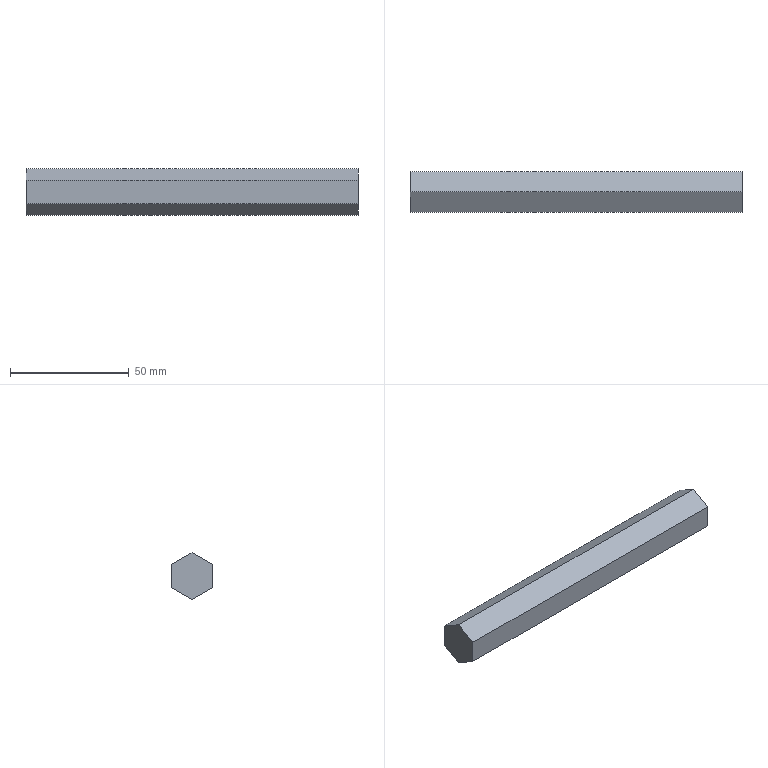Part | STEP file | JBJ-P-1002-09 | 1 solid | 8 faces | box 140 x 17 x 19.63 mm | volume 35039 mm3 | plane 8
STEP:
#1=CARTESIAN_POINT('',(0.,-8.5,4.907));
#2=VERTEX_POINT('',#1);
#3=CARTESIAN_POINT('',(0.,-8.5,-4.907));
#4=VERTEX_POINT('',#3);
#5=CARTESIAN_POINT('',(0.,-8.5,4.907));
#6=DIRECTION('',(0.,0.,-1.));
#7=VECTOR('',#6,1000.);
#8=LINE('',#5,#7);
#9=EDGE_CURVE('',#2,#4,#8,.T.);
#10=ORIENTED_EDGE('',*,*,#9,.T.);
#11=CARTESIAN_POINT('',(140.,-8.5,-4.907));
#12=VERTEX_POINT('',#11);
#13=CARTESIAN_POINT('',(140.,-8.5,-4.907));
#14=DIRECTION('',(-1.,0.,0.));
#15=VECTOR('',#14,1000.);
#16=LINE('',#13,#15);
#17=EDGE_CURVE('',#12,#4,#16,.T.);
#18=ORIENTED_EDGE('',*,*,#17,.F.);
#19=CARTESIAN_POINT('',(140.,-8.5,4.907));
#20=VERTEX_POINT('',#19);
#21=CARTESIAN_POINT('',(140.,-8.5,4.907));
#22=DIRECTION('',(0.,0.,-1.));
#23=VECTOR('',#22,1000.);
#24=LINE('',#21,#23);
#25=EDGE_CURVE('',#20,#12,#24,.T.);
#26=ORIENTED_EDGE('',*,*,#25,.F.);
#27=CARTESIAN_POINT('',(140.,-8.5,4.907));
#28=DIRECTION('',(-1.,0.,0.));
#29=VECTOR('',#28,1000.);
#30=LINE('',#27,#29);
#31=EDGE_CURVE('',#20,#2,#30,.T.);
#32=ORIENTED_EDGE('',*,*,#31,.T.);
#33=EDGE_LOOP('',(#10,#18,#26,#32));
#34=FACE_OUTER_BOUND('',#33,.T.);
#35=CARTESIAN_POINT('',(140.,-8.5,4.907));
#36=DIRECTION('',(0.,1.,0.));
#37=DIRECTION('',(0.,0.,1.));
#38=AXIS2_PLACEMENT_3D('',#35,#36,#37);
#39=PLANE('',#38);
#40=ADVANCED_FACE('',(#34),#39,.F.);
#41=CARTESIAN_POINT('',(0.,0.,-9.815));
#42=VERTEX_POINT('',#41);
#43=CARTESIAN_POINT('',(0.,-8.5,-4.907));
#44=DIRECTION('',(0.,0.866,-0.5));
#45=VECTOR('',#44,1000.);
#46=LINE('',#43,#45);
#47=EDGE_CURVE('',#4,#42,#46,.T.);
#48=ORIENTED_EDGE('',*,*,#47,.T.);
#49=CARTESIAN_POINT('',(140.,0.,-9.815));
#50=VERTEX_POINT('',#49);
#51=CARTESIAN_POINT('',(140.,0.,-9.815));
#52=DIRECTION('',(-1.,0.,0.));
#53=VECTOR('',#52,1000.);
#54=LINE('',#51,#53);
#55=EDGE_CURVE('',#50,#42,#54,.T.);
#56=ORIENTED_EDGE('',*,*,#55,.F.);
#57=CARTESIAN_POINT('',(140.,-8.5,-4.907));
#58=DIRECTION('',(0.,0.866,-0.5));
#59=VECTOR('',#58,1000.);
#60=LINE('',#57,#59);
#61=EDGE_CURVE('',#12,#50,#60,.T.);
#62=ORIENTED_EDGE('',*,*,#61,.F.);
#63=ORIENTED_EDGE('',*,*,#17,.T.);
#64=EDGE_LOOP('',(#48,#56,#62,#63));
#65=FACE_OUTER_BOUND('',#64,.T.);
#66=CARTESIAN_POINT('',(140.,-8.5,-4.907));
#67=DIRECTION('',(0.,0.5,0.866));
#68=DIRECTION('',(0.,-0.866,0.5));
#69=AXIS2_PLACEMENT_3D('',#66,#67,#68);
#70=PLANE('',#69);
#71=ADVANCED_FACE('',(#65),#70,.F.);
#72=CARTESIAN_POINT('',(0.,8.5,-4.907));
#73=VERTEX_POINT('',#72);
#74=CARTESIAN_POINT('',(0.,0.,-9.815));
#75=DIRECTION('',(0.,0.866,0.5));
#76=VECTOR('',#75,1000.);
#77=LINE('',#74,#76);
#78=EDGE_CURVE('',#42,#73,#77,.T.);
#79=ORIENTED_EDGE('',*,*,#78,.T.);
#80=CARTESIAN_POINT('',(140.,8.5,-4.907));
#81=VERTEX_POINT('',#80);
#82=CARTESIAN_POINT('',(140.,8.5,-4.907));
#83=DIRECTION('',(-1.,0.,0.));
#84=VECTOR('',#83,1000.);
#85=LINE('',#82,#84);
#86=EDGE_CURVE('',#81,#73,#85,.T.);
#87=ORIENTED_EDGE('',*,*,#86,.F.);
#88=CARTESIAN_POINT('',(140.,0.,-9.815));
#89=DIRECTION('',(0.,0.866,0.5));
#90=VECTOR('',#89,1000.);
#91=LINE('',#88,#90);
#92=EDGE_CURVE('',#50,#81,#91,.T.);
#93=ORIENTED_EDGE('',*,*,#92,.F.);
#94=ORIENTED_EDGE('',*,*,#55,.T.);
#95=EDGE_LOOP('',(#79,#87,#93,#94));
#96=FACE_OUTER_BOUND('',#95,.T.);
#97=CARTESIAN_POINT('',(140.,0.,-9.815));
#98=DIRECTION('',(0.,-0.5,0.866));
#99=DIRECTION('',(0.,-0.866,-0.5));
#100=AXIS2_PLACEMENT_3D('',#97,#98,#99);
#101=PLANE('',#100);
#102=ADVANCED_FACE('',(#96),#101,.F.);
#103=CARTESIAN_POINT('',(0.,8.5,4.907));
#104=VERTEX_POINT('',#103);
#105=CARTESIAN_POINT('',(0.,8.5,-4.907));
#106=DIRECTION('',(0.,0.,1.));
#107=VECTOR('',#106,1000.);
#108=LINE('',#105,#107);
#109=EDGE_CURVE('',#73,#104,#108,.T.);
#110=ORIENTED_EDGE('',*,*,#109,.T.);
#111=CARTESIAN_POINT('',(140.,8.5,4.907));
#112=VERTEX_POINT('',#111);
#113=CARTESIAN_POINT('',(140.,8.5,4.907));
#114=DIRECTION('',(-1.,0.,0.));
#115=VECTOR('',#114,1000.);
#116=LINE('',#113,#115);
#117=EDGE_CURVE('',#112,#104,#116,.T.);
#118=ORIENTED_EDGE('',*,*,#117,.F.);
#119=CARTESIAN_POINT('',(140.,8.5,-4.907));
#120=DIRECTION('',(0.,0.,1.));
#121=VECTOR('',#120,1000.);
#122=LINE('',#119,#121);
#123=EDGE_CURVE('',#81,#112,#122,.T.);
#124=ORIENTED_EDGE('',*,*,#123,.F.);
#125=ORIENTED_EDGE('',*,*,#86,.T.);
#126=EDGE_LOOP('',(#110,#118,#124,#125));
#127=FACE_OUTER_BOUND('',#126,.T.);
#128=CARTESIAN_POINT('',(140.,8.5,-4.907));
#129=DIRECTION('',(0.,-1.,0.));
#130=DIRECTION('',(0.,0.,-1.));
#131=AXIS2_PLACEMENT_3D('',#128,#129,#130);
#132=PLANE('',#131);
#133=ADVANCED_FACE('',(#127),#132,.F.);
#134=CARTESIAN_POINT('',(0.,0.,9.815));
#135=VERTEX_POINT('',#134);
#136=CARTESIAN_POINT('',(0.,8.5,4.907));
#137=DIRECTION('',(0.,-0.866,0.5));
#138=VECTOR('',#137,1000.);
#139=LINE('',#136,#138);
#140=EDGE_CURVE('',#104,#135,#139,.T.);
#141=ORIENTED_EDGE('',*,*,#140,.T.);
#142=CARTESIAN_POINT('',(140.,0.,9.815));
#143=VERTEX_POINT('',#142);
#144=CARTESIAN_POINT('',(140.,0.,9.815));
#145=DIRECTION('',(-1.,0.,0.));
#146=VECTOR('',#145,1000.);
#147=LINE('',#144,#146);
#148=EDGE_CURVE('',#143,#135,#147,.T.);
#149=ORIENTED_EDGE('',*,*,#148,.F.);
#150=CARTESIAN_POINT('',(140.,8.5,4.907));
#151=DIRECTION('',(0.,-0.866,0.5));
#152=VECTOR('',#151,1000.);
#153=LINE('',#150,#152);
#154=EDGE_CURVE('',#112,#143,#153,.T.);
#155=ORIENTED_EDGE('',*,*,#154,.F.);
#156=ORIENTED_EDGE('',*,*,#117,.T.);
#157=EDGE_LOOP('',(#141,#149,#155,#156));
#158=FACE_OUTER_BOUND('',#157,.T.);
#159=CARTESIAN_POINT('',(140.,8.5,4.907));
#160=DIRECTION('',(0.,-0.5,-0.866));
#161=DIRECTION('',(0.,0.866,-0.5));
#162=AXIS2_PLACEMENT_3D('',#159,#160,#161);
#163=PLANE('',#162);
#164=ADVANCED_FACE('',(#158),#163,.F.);
#165=CARTESIAN_POINT('',(0.,0.,9.815));
#166=DIRECTION('',(0.,-0.866,-0.5));
#167=VECTOR('',#166,1000.);
#168=LINE('',#165,#167);
#169=EDGE_CURVE('',#135,#2,#168,.T.);
#170=ORIENTED_EDGE('',*,*,#169,.T.);
#171=ORIENTED_EDGE('',*,*,#31,.F.);
#172=CARTESIAN_POINT('',(140.,0.,9.815));
#173=DIRECTION('',(0.,-0.866,-0.5));
#174=VECTOR('',#173,1000.);
#175=LINE('',#172,#174);
#176=EDGE_CURVE('',#143,#20,#175,.T.);
#177=ORIENTED_EDGE('',*,*,#176,.F.);
#178=ORIENTED_EDGE('',*,*,#148,.T.);
#179=EDGE_LOOP('',(#170,#171,#177,#178));
#180=FACE_OUTER_BOUND('',#179,.T.);
#181=CARTESIAN_POINT('',(140.,0.,9.815));
#182=DIRECTION('',(0.,0.5,-0.866));
#183=DIRECTION('',(0.,0.866,0.5));
#184=AXIS2_PLACEMENT_3D('',#181,#182,#183);
#185=PLANE('',#184);
#186=ADVANCED_FACE('',(#180),#185,.F.);
#187=ORIENTED_EDGE('',*,*,#25,.T.);
#188=ORIENTED_EDGE('',*,*,#61,.T.);
#189=ORIENTED_EDGE('',*,*,#92,.T.);
#190=ORIENTED_EDGE('',*,*,#123,.T.);
#191=ORIENTED_EDGE('',*,*,#154,.T.);
#192=ORIENTED_EDGE('',*,*,#176,.T.);
#193=EDGE_LOOP('',(#187,#188,#189,#190,#191,#192));
#194=FACE_OUTER_BOUND('',#193,.T.);
#195=CARTESIAN_POINT('',(140.,0.,0.));
#196=DIRECTION('',(1.,0.,0.));
#197=DIRECTION('',(0.,0.,-1.));
#198=AXIS2_PLACEMENT_3D('',#195,#196,#197);
#199=PLANE('',#198);
#200=ADVANCED_FACE('',(#194),#199,.T.);
#201=ORIENTED_EDGE('',*,*,#9,.F.);
#202=ORIENTED_EDGE('',*,*,#169,.F.);
#203=ORIENTED_EDGE('',*,*,#140,.F.);
#204=ORIENTED_EDGE('',*,*,#109,.F.);
#205=ORIENTED_EDGE('',*,*,#78,.F.);
#206=ORIENTED_EDGE('',*,*,#47,.F.);
#207=EDGE_LOOP('',(#201,#202,#203,#204,#205,#206));
#208=FACE_OUTER_BOUND('',#207,.T.);
#209=CARTESIAN_POINT('',(0.,0.,0.));
#210=DIRECTION('',(1.,0.,0.));
#211=DIRECTION('',(0.,0.,-1.));
#212=AXIS2_PLACEMENT_3D('',#209,#210,#211);
#213=PLANE('',#212);
#214=ADVANCED_FACE('',(#208),#213,.F.);
#215=CLOSED_SHELL('',(#40,#71,#102,#133,#164,#186,#200,#214));
#216=MANIFOLD_SOLID_BREP('',#215);
#217=CARTESIAN_POINT('',(0.,0.,0.));
#218=DIRECTION('',(0.,0.,1.));
#219=DIRECTION('',(1.,0.,0.));
#220=AXIS2_PLACEMENT_3D('',#217,#218,#219);
#221=(LENGTH_UNIT()NAMED_UNIT(*)SI_UNIT(.MILLI.,.METRE.));
#222=UNCERTAINTY_MEASURE_WITH_UNIT(LENGTH_MEASURE(0.00001),#221,'','');
#223=(NAMED_UNIT(*)PLANE_ANGLE_UNIT()SI_UNIT($,.RADIAN.));
#224=(NAMED_UNIT(*)SI_UNIT($,.STERADIAN.)SOLID_ANGLE_UNIT());
#225=(GEOMETRIC_REPRESENTATION_CONTEXT(3)GLOBAL_UNCERTAINTY_ASSIGNED_CONTEXT((#222))GLOBAL_UNIT_ASSIGNED_CONTEXT((#221,#223,#224))REPRESENTATION_CONTEXT('',''));
#226=ADVANCED_BREP_SHAPE_REPRESENTATION('',(#216,#220),#225);